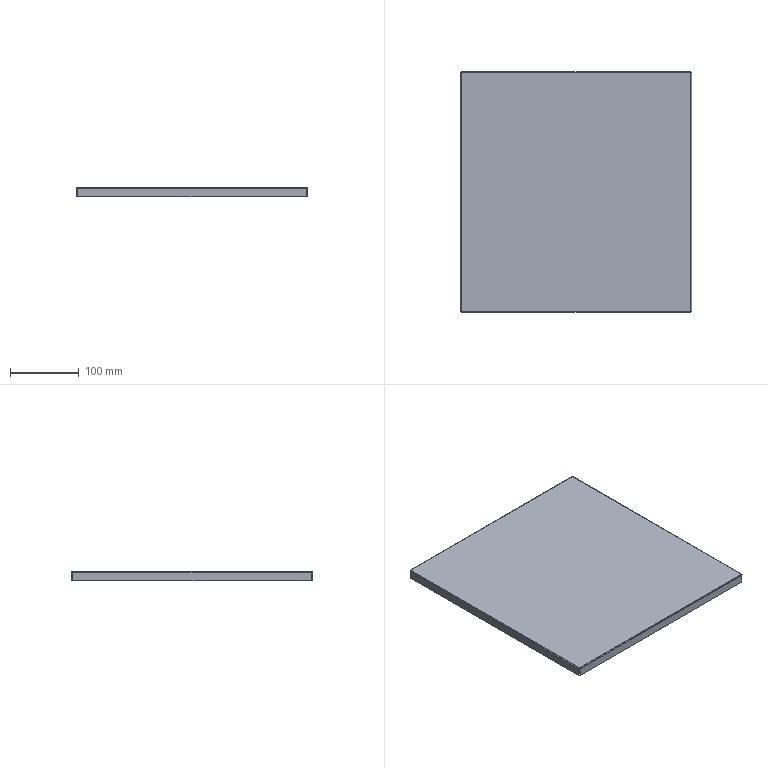Part | STEP file | Electrical plate | 1 solid | 38 faces | box 337.193 x 351.476 x 13.2 mm | volume 161258 mm3 | plane 22 | spline 8 | cylinder 8 | commonest cylinder face diameters 0.4 x4 2.8 x4
STEP:
#1=CARTESIAN_POINT('',(167.196,-174.338,-1.2));
#2=VERTEX_POINT('',#1);
#3=CARTESIAN_POINT('',(167.196,174.338,-1.2));
#4=VERTEX_POINT('',#3);
#5=CARTESIAN_POINT('',(167.196,-174.338,-1.2));
#6=DIRECTION('',(0.,1.,0.));
#7=VECTOR('',#6,1000.);
#8=LINE('',#5,#7);
#9=EDGE_CURVE('',#2,#4,#8,.T.);
#10=ORIENTED_EDGE('',*,*,#9,.F.);
#11=CARTESIAN_POINT('',(-167.196,-174.338,-1.2));
#12=VERTEX_POINT('',#11);
#13=CARTESIAN_POINT('',(-167.196,-174.338,-1.2));
#14=DIRECTION('',(1.,0.,0.));
#15=VECTOR('',#14,1000.);
#16=LINE('',#13,#15);
#17=EDGE_CURVE('',#12,#2,#16,.T.);
#18=ORIENTED_EDGE('',*,*,#17,.F.);
#19=CARTESIAN_POINT('',(-167.196,174.338,-1.2));
#20=VERTEX_POINT('',#19);
#21=CARTESIAN_POINT('',(-167.196,174.338,-1.2));
#22=DIRECTION('',(0.,-1.,0.));
#23=VECTOR('',#22,1000.);
#24=LINE('',#21,#23);
#25=EDGE_CURVE('',#20,#12,#24,.T.);
#26=ORIENTED_EDGE('',*,*,#25,.F.);
#27=CARTESIAN_POINT('',(167.196,174.338,-1.2));
#28=DIRECTION('',(-1.,0.,0.));
#29=VECTOR('',#28,1000.);
#30=LINE('',#27,#29);
#31=EDGE_CURVE('',#4,#20,#30,.T.);
#32=ORIENTED_EDGE('',*,*,#31,.F.);
#33=EDGE_LOOP('',(#10,#18,#26,#32));
#34=FACE_OUTER_BOUND('',#33,.T.);
#35=CARTESIAN_POINT('',(0.,0.,-1.2));
#36=DIRECTION('',(0.,0.,-1.));
#37=DIRECTION('',(-1.,0.,0.));
#38=AXIS2_PLACEMENT_3D('',#35,#36,#37);
#39=PLANE('',#38);
#40=ADVANCED_FACE('',(#34),#39,.T.);
#41=CARTESIAN_POINT('',(-167.196,-174.338,0.));
#42=VERTEX_POINT('',#41);
#43=CARTESIAN_POINT('',(167.196,-174.338,0.));
#44=VERTEX_POINT('',#43);
#45=CARTESIAN_POINT('',(-167.196,-174.338,0.));
#46=DIRECTION('',(1.,0.,0.));
#47=VECTOR('',#46,1000.);
#48=LINE('',#45,#47);
#49=EDGE_CURVE('',#42,#44,#48,.T.);
#50=ORIENTED_EDGE('',*,*,#49,.T.);
#51=CARTESIAN_POINT('',(167.196,174.338,0.));
#52=VERTEX_POINT('',#51);
#53=CARTESIAN_POINT('',(167.196,-174.338,0.));
#54=DIRECTION('',(0.,1.,0.));
#55=VECTOR('',#54,1000.);
#56=LINE('',#53,#55);
#57=EDGE_CURVE('',#44,#52,#56,.T.);
#58=ORIENTED_EDGE('',*,*,#57,.T.);
#59=CARTESIAN_POINT('',(-167.196,174.338,0.));
#60=VERTEX_POINT('',#59);
#61=CARTESIAN_POINT('',(167.196,174.338,0.));
#62=DIRECTION('',(-1.,0.,0.));
#63=VECTOR('',#62,1000.);
#64=LINE('',#61,#63);
#65=EDGE_CURVE('',#52,#60,#64,.T.);
#66=ORIENTED_EDGE('',*,*,#65,.T.);
#67=CARTESIAN_POINT('',(-167.196,174.338,0.));
#68=DIRECTION('',(0.,-1.,0.));
#69=VECTOR('',#68,1000.);
#70=LINE('',#67,#69);
#71=EDGE_CURVE('',#60,#42,#70,.T.);
#72=ORIENTED_EDGE('',*,*,#71,.T.);
#73=EDGE_LOOP('',(#50,#58,#66,#72));
#74=FACE_OUTER_BOUND('',#73,.T.);
#75=CARTESIAN_POINT('',(0.,0.,0.));
#76=DIRECTION('',(0.,0.,-1.));
#77=DIRECTION('',(-1.,0.,0.));
#78=AXIS2_PLACEMENT_3D('',#75,#76,#77);
#79=PLANE('',#78);
#80=ADVANCED_FACE('',(#74),#79,.F.);
#81=CARTESIAN_POINT('',(-168.596,-173.831,-1.4));
#82=VERTEX_POINT('',#81);
#83=CARTESIAN_POINT('',(-167.396,-173.831,-1.4));
#84=VERTEX_POINT('',#83);
#85=CARTESIAN_POINT('',(-167.396,-173.831,-1.4));
#86=DIRECTION('',(1.,0.,0.));
#87=VECTOR('',#86,1000.);
#88=LINE('',#85,#87);
#89=EDGE_CURVE('',#82,#84,#88,.T.);
#90=ORIENTED_EDGE('',*,*,#89,.T.);
#91=CARTESIAN_POINT('',(-167.196,-174.338,-1.2));
#92=CARTESIAN_POINT('',(-167.249,-174.254,-1.2));
#93=CARTESIAN_POINT('',(-167.301,-174.169,-1.222));
#94=CARTESIAN_POINT('',(-167.375,-174.,-1.296));
#95=CARTESIAN_POINT('',(-167.396,-173.916,-1.348));
#96=CARTESIAN_POINT('',(-167.396,-173.831,-1.4));
#97=B_SPLINE_CURVE_WITH_KNOTS('',3,(#91,#92,#93,#94,#95,#96),.UNSPECIFIED.,.F.,.F.,(4,2,4),(0.,0.5,1.),.UNSPECIFIED.);
#98=EDGE_CURVE('',#12,#84,#97,.T.);
#99=ORIENTED_EDGE('',*,*,#98,.F.);
#100=CARTESIAN_POINT('',(-167.196,-174.338,-1.2));
#101=DIRECTION('',(0.,0.,1.));
#102=VECTOR('',#101,1000.);
#103=LINE('',#100,#102);
#104=EDGE_CURVE('',#12,#42,#103,.T.);
#105=ORIENTED_EDGE('',*,*,#104,.T.);
#106=CARTESIAN_POINT('',(-167.196,-174.338,0.));
#107=CARTESIAN_POINT('',(-167.38,-174.296,0.));
#108=CARTESIAN_POINT('',(-167.563,-174.254,-0.03644));
#109=CARTESIAN_POINT('',(-167.901,-174.169,-0.1767));
#110=CARTESIAN_POINT('',(-168.057,-174.127,-0.2805));
#111=CARTESIAN_POINT('',(-168.316,-174.042,-0.5396));
#112=CARTESIAN_POINT('',(-168.42,-174.,-0.6949));
#113=CARTESIAN_POINT('',(-168.56,-173.916,-1.034));
#114=CARTESIAN_POINT('',(-168.596,-173.873,-1.217));
#115=CARTESIAN_POINT('',(-168.596,-173.831,-1.4));
#116=B_SPLINE_CURVE_WITH_KNOTS('',3,(#106,#107,#108,#109,#110,#111,#112,#113,#114,#115),.UNSPECIFIED.,.F.,.F.,(4,2,2,2,4),(0.,0.25,0.5,0.75,1.),.UNSPECIFIED.);
#117=EDGE_CURVE('',#42,#82,#116,.T.);
#118=ORIENTED_EDGE('',*,*,#117,.T.);
#119=EDGE_LOOP('',(#90,#99,#105,#118));
#120=FACE_OUTER_BOUND('',#119,.T.);
#121=CARTESIAN_POINT('',(-167.196,-174.338,0.012));
#122=CARTESIAN_POINT('',(-167.381,-174.296,0.012));
#123=CARTESIAN_POINT('',(-167.566,-174.254,-0.02475));
#124=CARTESIAN_POINT('',(-167.907,-174.169,-0.1662));
#125=CARTESIAN_POINT('',(-168.064,-174.127,-0.2709));
#126=CARTESIAN_POINT('',(-168.325,-174.042,-0.5323));
#127=CARTESIAN_POINT('',(-168.43,-174.,-0.6889));
#128=CARTESIAN_POINT('',(-168.572,-173.916,-1.03));
#129=CARTESIAN_POINT('',(-168.608,-173.873,-1.215));
#130=CARTESIAN_POINT('',(-168.608,-173.831,-1.4));
#131=CARTESIAN_POINT('',(-167.196,-174.338,0.));
#132=CARTESIAN_POINT('',(-167.38,-174.296,0.));
#133=CARTESIAN_POINT('',(-167.563,-174.254,-0.03644));
#134=CARTESIAN_POINT('',(-167.901,-174.169,-0.1767));
#135=CARTESIAN_POINT('',(-168.057,-174.127,-0.2805));
#136=CARTESIAN_POINT('',(-168.316,-174.042,-0.5396));
#137=CARTESIAN_POINT('',(-168.42,-174.,-0.6949));
#138=CARTESIAN_POINT('',(-168.56,-173.916,-1.034));
#139=CARTESIAN_POINT('',(-168.596,-173.873,-1.217));
#140=CARTESIAN_POINT('',(-168.596,-173.831,-1.4));
#141=CARTESIAN_POINT('',(-167.196,-174.338,-1.2));
#142=CARTESIAN_POINT('',(-167.222,-174.296,-1.2));
#143=CARTESIAN_POINT('',(-167.249,-174.254,-1.205));
#144=CARTESIAN_POINT('',(-167.297,-174.169,-1.225));
#145=CARTESIAN_POINT('',(-167.319,-174.127,-1.24));
#146=CARTESIAN_POINT('',(-167.356,-174.042,-1.277));
#147=CARTESIAN_POINT('',(-167.371,-174.,-1.299));
#148=CARTESIAN_POINT('',(-167.391,-173.916,-1.348));
#149=CARTESIAN_POINT('',(-167.396,-173.873,-1.374));
#150=CARTESIAN_POINT('',(-167.396,-173.831,-1.4));
#151=CARTESIAN_POINT('',(-167.196,-174.338,-1.212));
#152=CARTESIAN_POINT('',(-167.221,-174.296,-1.212));
#153=CARTESIAN_POINT('',(-167.245,-174.254,-1.217));
#154=CARTESIAN_POINT('',(-167.291,-174.169,-1.236));
#155=CARTESIAN_POINT('',(-167.312,-174.127,-1.25));
#156=CARTESIAN_POINT('',(-167.347,-174.042,-1.285));
#157=CARTESIAN_POINT('',(-167.36,-174.,-1.305));
#158=CARTESIAN_POINT('',(-167.379,-173.916,-1.351));
#159=CARTESIAN_POINT('',(-167.384,-173.873,-1.375));
#160=CARTESIAN_POINT('',(-167.384,-173.831,-1.4));
#161=B_SPLINE_SURFACE_WITH_KNOTS('',1,3,((#121,#122,#123,#124,#125,#126,#127,#128,#129,#130),(#131,#132,#133,#134,#135,#136,#137,#138,#139,#140),(#141,#142,#143,#144,#145,#146,#147,#148,#149,#150),(#151,#152,#153,#154,#155,#156,#157,#158,#159,#160)),.UNSPECIFIED.,.F.,.F.,.F.,(2,1,1,2),(4,2,2,2,4),(-0.01,0.,1.,1.01),(0.,0.25,0.5,0.75,1.),.UNSPECIFIED.);
#162=ADVANCED_FACE('',(#120),#161,.F.);
#163=CARTESIAN_POINT('',(-167.396,173.831,-1.4));
#164=VERTEX_POINT('',#163);
#165=CARTESIAN_POINT('',(-167.396,173.831,-1.4));
#166=CARTESIAN_POINT('',(-167.396,173.916,-1.348));
#167=CARTESIAN_POINT('',(-167.375,174.,-1.296));
#168=CARTESIAN_POINT('',(-167.301,174.169,-1.222));
#169=CARTESIAN_POINT('',(-167.249,174.254,-1.2));
#170=CARTESIAN_POINT('',(-167.196,174.338,-1.2));
#171=B_SPLINE_CURVE_WITH_KNOTS('',3,(#165,#166,#167,#168,#169,#170),.UNSPECIFIED.,.F.,.F.,(4,2,4),(0.,0.5,1.),.UNSPECIFIED.);
#172=EDGE_CURVE('',#164,#20,#171,.T.);
#173=ORIENTED_EDGE('',*,*,#172,.F.);
#174=CARTESIAN_POINT('',(-168.596,173.831,-1.4));
#175=VERTEX_POINT('',#174);
#176=CARTESIAN_POINT('',(-167.396,173.831,-1.4));
#177=DIRECTION('',(1.,0.,0.));
#178=VECTOR('',#177,1000.);
#179=LINE('',#176,#178);
#180=EDGE_CURVE('',#175,#164,#179,.T.);
#181=ORIENTED_EDGE('',*,*,#180,.F.);
#182=CARTESIAN_POINT('',(-168.596,173.831,-1.4));
#183=CARTESIAN_POINT('',(-168.596,173.873,-1.217));
#184=CARTESIAN_POINT('',(-168.56,173.916,-1.034));
#185=CARTESIAN_POINT('',(-168.42,174.,-0.6949));
#186=CARTESIAN_POINT('',(-168.316,174.042,-0.5396));
#187=CARTESIAN_POINT('',(-168.057,174.127,-0.2805));
#188=CARTESIAN_POINT('',(-167.901,174.169,-0.1767));
#189=CARTESIAN_POINT('',(-167.563,174.254,-0.03644));
#190=CARTESIAN_POINT('',(-167.38,174.296,0.));
#191=CARTESIAN_POINT('',(-167.196,174.338,0.));
#192=B_SPLINE_CURVE_WITH_KNOTS('',3,(#182,#183,#184,#185,#186,#187,#188,#189,#190,#191),.UNSPECIFIED.,.F.,.F.,(4,2,2,2,4),(0.,0.25,0.5,0.75,1.),.UNSPECIFIED.);
#193=EDGE_CURVE('',#175,#60,#192,.T.);
#194=ORIENTED_EDGE('',*,*,#193,.T.);
#195=CARTESIAN_POINT('',(-167.196,174.338,-1.2));
#196=DIRECTION('',(0.,0.,1.));
#197=VECTOR('',#196,1000.);
#198=LINE('',#195,#197);
#199=EDGE_CURVE('',#20,#60,#198,.T.);
#200=ORIENTED_EDGE('',*,*,#199,.F.);
#201=EDGE_LOOP('',(#173,#181,#194,#200));
#202=FACE_OUTER_BOUND('',#201,.T.);
#203=CARTESIAN_POINT('',(-168.608,173.831,-1.4));
#204=CARTESIAN_POINT('',(-168.608,173.873,-1.215));
#205=CARTESIAN_POINT('',(-168.572,173.916,-1.03));
#206=CARTESIAN_POINT('',(-168.43,174.,-0.6889));
#207=CARTESIAN_POINT('',(-168.325,174.042,-0.5323));
#208=CARTESIAN_POINT('',(-168.064,174.127,-0.2709));
#209=CARTESIAN_POINT('',(-167.907,174.169,-0.1662));
#210=CARTESIAN_POINT('',(-167.566,174.254,-0.02475));
#211=CARTESIAN_POINT('',(-167.381,174.296,0.012));
#212=CARTESIAN_POINT('',(-167.196,174.338,0.012));
#213=CARTESIAN_POINT('',(-168.596,173.831,-1.4));
#214=CARTESIAN_POINT('',(-168.596,173.873,-1.217));
#215=CARTESIAN_POINT('',(-168.56,173.916,-1.034));
#216=CARTESIAN_POINT('',(-168.42,174.,-0.6949));
#217=CARTESIAN_POINT('',(-168.316,174.042,-0.5396));
#218=CARTESIAN_POINT('',(-168.057,174.127,-0.2805));
#219=CARTESIAN_POINT('',(-167.901,174.169,-0.1767));
#220=CARTESIAN_POINT('',(-167.563,174.254,-0.03644));
#221=CARTESIAN_POINT('',(-167.38,174.296,0.));
#222=CARTESIAN_POINT('',(-167.196,174.338,0.));
#223=CARTESIAN_POINT('',(-167.396,173.831,-1.4));
#224=CARTESIAN_POINT('',(-167.396,173.873,-1.374));
#225=CARTESIAN_POINT('',(-167.391,173.916,-1.348));
#226=CARTESIAN_POINT('',(-167.371,174.,-1.299));
#227=CARTESIAN_POINT('',(-167.356,174.042,-1.277));
#228=CARTESIAN_POINT('',(-167.319,174.127,-1.24));
#229=CARTESIAN_POINT('',(-167.297,174.169,-1.225));
#230=CARTESIAN_POINT('',(-167.249,174.254,-1.205));
#231=CARTESIAN_POINT('',(-167.222,174.296,-1.2));
#232=CARTESIAN_POINT('',(-167.196,174.338,-1.2));
#233=CARTESIAN_POINT('',(-167.384,173.831,-1.4));
#234=CARTESIAN_POINT('',(-167.384,173.873,-1.375));
#235=CARTESIAN_POINT('',(-167.379,173.916,-1.351));
#236=CARTESIAN_POINT('',(-167.36,174.,-1.305));
#237=CARTESIAN_POINT('',(-167.347,174.042,-1.285));
#238=CARTESIAN_POINT('',(-167.312,174.127,-1.25));
#239=CARTESIAN_POINT('',(-167.291,174.169,-1.236));
#240=CARTESIAN_POINT('',(-167.245,174.254,-1.217));
#241=CARTESIAN_POINT('',(-167.221,174.296,-1.212));
#242=CARTESIAN_POINT('',(-167.196,174.338,-1.212));
#243=B_SPLINE_SURFACE_WITH_KNOTS('',1,3,((#203,#204,#205,#206,#207,#208,#209,#210,#211,#212),(#213,#214,#215,#216,#217,#218,#219,#220,#221,#222),(#223,#224,#225,#226,#227,#228,#229,#230,#231,#232),(#233,#234,#235,#236,#237,#238,#239,#240,#241,#242)),.UNSPECIFIED.,.F.,.F.,.F.,(2,1,1,2),(4,2,2,2,4),(-0.01,0.,1.,1.01),(0.,0.25,0.5,0.75,1.),.UNSPECIFIED.);
#244=ADVANCED_FACE('',(#202),#243,.F.);
#245=ORIENTED_EDGE('',*,*,#71,.F.);
#246=ORIENTED_EDGE('',*,*,#193,.F.);
#247=CARTESIAN_POINT('',(-168.596,0.,-1.4));
#248=DIRECTION('',(0.,1.,0.));
#249=VECTOR('',#248,1000.);
#250=LINE('',#247,#249);
#251=EDGE_CURVE('',#82,#175,#250,.T.);
#252=ORIENTED_EDGE('',*,*,#251,.F.);
#253=ORIENTED_EDGE('',*,*,#117,.F.);
#254=EDGE_LOOP('',(#245,#246,#252,#253));
#255=FACE_OUTER_BOUND('',#254,.T.);
#256=CARTESIAN_POINT('',(-167.196,174.338,-1.4));
#257=DIRECTION('',(0.,1.,0.));
#258=DIRECTION('',(-1.,0.,0.));
#259=AXIS2_PLACEMENT_3D('',#256,#257,#258);
#260=CYLINDRICAL_SURFACE('',#259,1.4);
#261=ADVANCED_FACE('',(#255),#260,.T.);
#262=ORIENTED_EDGE('',*,*,#25,.T.);
#263=ORIENTED_EDGE('',*,*,#98,.T.);
#264=CARTESIAN_POINT('',(-167.396,-174.538,-1.4));
#265=DIRECTION('',(0.,1.,0.));
#266=VECTOR('',#265,1000.);
#267=LINE('',#264,#266);
#268=EDGE_CURVE('',#84,#164,#267,.T.);
#269=ORIENTED_EDGE('',*,*,#268,.T.);
#270=ORIENTED_EDGE('',*,*,#172,.T.);
#271=EDGE_LOOP('',(#262,#263,#269,#270));
#272=FACE_OUTER_BOUND('',#271,.T.);
#273=CARTESIAN_POINT('',(-167.196,174.338,-1.4));
#274=DIRECTION('',(0.,1.,0.));
#275=DIRECTION('',(-1.,0.,0.));
#276=AXIS2_PLACEMENT_3D('',#273,#274,#275);
#277=CYLINDRICAL_SURFACE('',#276,0.2);
#278=ADVANCED_FACE('',(#272),#277,.F.);
#279=CARTESIAN_POINT('',(-167.396,-173.831,-13.2));
#280=VERTEX_POINT('',#279);
#281=CARTESIAN_POINT('',(-168.596,-173.831,-13.2));
#282=VERTEX_POINT('',#281);
#283=CARTESIAN_POINT('',(-168.596,-173.831,-13.2));
#284=DIRECTION('',(-1.,0.,0.));
#285=VECTOR('',#284,1000.);
#286=LINE('',#283,#285);
#287=EDGE_CURVE('',#280,#282,#286,.T.);
#288=ORIENTED_EDGE('',*,*,#287,.F.);
#289=CARTESIAN_POINT('',(-167.396,-173.831,-1.2));
#290=DIRECTION('',(0.,0.,-1.));
#291=VECTOR('',#290,1000.);
#292=LINE('',#289,#291);
#293=EDGE_CURVE('',#84,#280,#292,.T.);
#294=ORIENTED_EDGE('',*,*,#293,.F.);
#295=ORIENTED_EDGE('',*,*,#89,.F.);
#296=CARTESIAN_POINT('',(-168.596,-173.831,0.));
#297=DIRECTION('',(0.,0.,1.));
#298=VECTOR('',#297,1000.);
#299=LINE('',#296,#298);
#300=EDGE_CURVE('',#282,#82,#299,.T.);
#301=ORIENTED_EDGE('',*,*,#300,.F.);
#302=EDGE_LOOP('',(#288,#294,#295,#301));
#303=FACE_OUTER_BOUND('',#302,.T.);
#304=CARTESIAN_POINT('',(-167.396,-173.831,-1.2));
#305=DIRECTION('',(0.,-1.,0.));
#306=DIRECTION('',(0.,0.,-1.));
#307=AXIS2_PLACEMENT_3D('',#304,#305,#306);
#308=PLANE('',#307);
#309=ADVANCED_FACE('',(#303),#308,.T.);
#310=CARTESIAN_POINT('',(-168.596,173.831,-13.2));
#311=VERTEX_POINT('',#310);
#312=CARTESIAN_POINT('',(-168.596,173.831,0.));
#313=DIRECTION('',(0.,0.,1.));
#314=VECTOR('',#313,1000.);
#315=LINE('',#312,#314);
#316=EDGE_CURVE('',#311,#175,#315,.T.);
#317=ORIENTED_EDGE('',*,*,#316,.F.);
#318=CARTESIAN_POINT('',(-168.596,174.538,-13.2));
#319=DIRECTION('',(0.,1.,0.));
#320=VECTOR('',#319,1000.);
#321=LINE('',#318,#320);
#322=EDGE_CURVE('',#282,#311,#321,.T.);
#323=ORIENTED_EDGE('',*,*,#322,.F.);
#324=ORIENTED_EDGE('',*,*,#300,.T.);
#325=ORIENTED_EDGE('',*,*,#251,.T.);
#326=EDGE_LOOP('',(#317,#323,#324,#325));
#327=FACE_OUTER_BOUND('',#326,.T.);
#328=CARTESIAN_POINT('',(-168.596,0.,0.));
#329=DIRECTION('',(-1.,0.,0.));
#330=DIRECTION('',(0.,0.,1.));
#331=AXIS2_PLACEMENT_3D('',#328,#329,#330);
#332=PLANE('',#331);
#333=ADVANCED_FACE('',(#327),#332,.T.);
#334=CARTESIAN_POINT('',(-167.396,173.831,-13.2));
#335=VERTEX_POINT('',#334);
#336=CARTESIAN_POINT('',(-167.396,174.538,-13.2));
#337=DIRECTION('',(0.,1.,0.));
#338=VECTOR('',#337,1000.);
#339=LINE('',#336,#338);
#340=EDGE_CURVE('',#280,#335,#339,.T.);
#341=ORIENTED_EDGE('',*,*,#340,.T.);
#342=CARTESIAN_POINT('',(-167.396,173.831,-1.2));
#343=DIRECTION('',(0.,0.,-1.));
#344=VECTOR('',#343,1000.);
#345=LINE('',#342,#344);
#346=EDGE_CURVE('',#164,#335,#345,.T.);
#347=ORIENTED_EDGE('',*,*,#346,.F.);
#348=ORIENTED_EDGE('',*,*,#268,.F.);
#349=ORIENTED_EDGE('',*,*,#293,.T.);
#350=EDGE_LOOP('',(#341,#347,#348,#349));
#351=FACE_OUTER_BOUND('',#350,.T.);
#352=CARTESIAN_POINT('',(-167.396,0.,0.));
#353=DIRECTION('',(-1.,0.,0.));
#354=DIRECTION('',(0.,0.,1.));
#355=AXIS2_PLACEMENT_3D('',#352,#353,#354);
#356=PLANE('',#355);
#357=ADVANCED_FACE('',(#351),#356,.F.);
#358=CARTESIAN_POINT('',(-168.596,173.831,-13.2));
#359=DIRECTION('',(-1.,0.,0.));
#360=VECTOR('',#359,1000.);
#361=LINE('',#358,#360);
#362=EDGE_CURVE('',#335,#311,#361,.T.);
#363=ORIENTED_EDGE('',*,*,#362,.F.);
#364=ORIENTED_EDGE('',*,*,#340,.F.);
#365=ORIENTED_EDGE('',*,*,#287,.T.);
#366=ORIENTED_EDGE('',*,*,#322,.T.);
#367=EDGE_LOOP('',(#363,#364,#365,#366));
#368=FACE_OUTER_BOUND('',#367,.T.);
#369=CARTESIAN_POINT('',(-168.596,174.538,-13.2));
#370=DIRECTION('',(0.,0.,-1.));
#371=DIRECTION('',(-1.,0.,0.));
#372=AXIS2_PLACEMENT_3D('',#369,#370,#371);
#373=PLANE('',#372);
#374=ADVANCED_FACE('',(#368),#373,.T.);
#375=ORIENTED_EDGE('',*,*,#346,.T.);
#376=ORIENTED_EDGE('',*,*,#362,.T.);
#377=ORIENTED_EDGE('',*,*,#316,.T.);
#378=ORIENTED_EDGE('',*,*,#180,.T.);
#379=EDGE_LOOP('',(#375,#376,#377,#378));
#380=FACE_OUTER_BOUND('',#379,.T.);
#381=CARTESIAN_POINT('',(-167.396,173.831,-1.2));
#382=DIRECTION('',(0.,-1.,0.));
#383=DIRECTION('',(0.,0.,-1.));
#384=AXIS2_PLACEMENT_3D('',#381,#382,#383);
#385=PLANE('',#384);
#386=ADVANCED_FACE('',(#380),#385,.F.);
#387=CARTESIAN_POINT('',(-166.689,175.738,-1.4));
#388=VERTEX_POINT('',#387);
#389=CARTESIAN_POINT('',(-166.689,174.538,-1.4));
#390=VERTEX_POINT('',#389);
#391=CARTESIAN_POINT('',(-166.689,174.538,-1.4));
#392=DIRECTION('',(0.,-1.,0.));
#393=VECTOR('',#392,1000.);
#394=LINE('',#391,#393);
#395=EDGE_CURVE('',#388,#390,#394,.T.);
#396=ORIENTED_EDGE('',*,*,#395,.T.);
#397=CARTESIAN_POINT('',(-167.196,174.338,-1.2));
#398=CARTESIAN_POINT('',(-167.112,174.39,-1.2));
#399=CARTESIAN_POINT('',(-167.027,174.443,-1.222));
#400=CARTESIAN_POINT('',(-166.858,174.517,-1.296));
#401=CARTESIAN_POINT('',(-166.774,174.538,-1.348));
#402=CARTESIAN_POINT('',(-166.689,174.538,-1.4));
#403=B_SPLINE_CURVE_WITH_KNOTS('',3,(#397,#398,#399,#400,#401,#402),.UNSPECIFIED.,.F.,.F.,(4,2,4),(0.,0.5,1.),.UNSPECIFIED.);
#404=EDGE_CURVE('',#20,#390,#403,.T.);
#405=ORIENTED_EDGE('',*,*,#404,.F.);
#406=ORIENTED_EDGE('',*,*,#199,.T.);
#407=CARTESIAN_POINT('',(-167.196,174.338,0.));
#408=CARTESIAN_POINT('',(-167.154,174.521,0.));
#409=CARTESIAN_POINT('',(-167.112,174.705,-0.03644));
#410=CARTESIAN_POINT('',(-167.027,175.043,-0.1767));
#411=CARTESIAN_POINT('',(-166.985,175.198,-0.2805));
#412=CARTESIAN_POINT('',(-166.9,175.458,-0.5396));
#413=CARTESIAN_POINT('',(-166.858,175.561,-0.6949));
#414=CARTESIAN_POINT('',(-166.774,175.702,-1.034));
#415=CARTESIAN_POINT('',(-166.731,175.738,-1.217));
#416=CARTESIAN_POINT('',(-166.689,175.738,-1.4));
#417=B_SPLINE_CURVE_WITH_KNOTS('',3,(#407,#408,#409,#410,#411,#412,#413,#414,#415,#416),.UNSPECIFIED.,.F.,.F.,(4,2,2,2,4),(0.,0.25,0.5,0.75,1.),.UNSPECIFIED.);
#418=EDGE_CURVE('',#60,#388,#417,.T.);
#419=ORIENTED_EDGE('',*,*,#418,.T.);
#420=EDGE_LOOP('',(#396,#405,#406,#419));
#421=FACE_OUTER_BOUND('',#420,.T.);
#422=CARTESIAN_POINT('',(-167.196,174.338,0.012));
#423=CARTESIAN_POINT('',(-167.154,174.523,0.012));
#424=CARTESIAN_POINT('',(-167.112,174.708,-0.02475));
#425=CARTESIAN_POINT('',(-167.027,175.049,-0.1662));
#426=CARTESIAN_POINT('',(-166.985,175.206,-0.2709));
#427=CARTESIAN_POINT('',(-166.9,175.467,-0.5323));
#428=CARTESIAN_POINT('',(-166.858,175.572,-0.6889));
#429=CARTESIAN_POINT('',(-166.774,175.713,-1.03));
#430=CARTESIAN_POINT('',(-166.731,175.75,-1.215));
#431=CARTESIAN_POINT('',(-166.689,175.75,-1.4));
#432=CARTESIAN_POINT('',(-167.196,174.338,0.));
#433=CARTESIAN_POINT('',(-167.154,174.521,0.));
#434=CARTESIAN_POINT('',(-167.112,174.705,-0.03644));
#435=CARTESIAN_POINT('',(-167.027,175.043,-0.1767));
#436=CARTESIAN_POINT('',(-166.985,175.198,-0.2805));
#437=CARTESIAN_POINT('',(-166.9,175.458,-0.5396));
#438=CARTESIAN_POINT('',(-166.858,175.561,-0.6949));
#439=CARTESIAN_POINT('',(-166.774,175.702,-1.034));
#440=CARTESIAN_POINT('',(-166.731,175.738,-1.217));
#441=CARTESIAN_POINT('',(-166.689,175.738,-1.4));
#442=CARTESIAN_POINT('',(-167.196,174.338,-1.2));
#443=CARTESIAN_POINT('',(-167.154,174.364,-1.2));
#444=CARTESIAN_POINT('',(-167.112,174.39,-1.205));
#445=CARTESIAN_POINT('',(-167.027,174.439,-1.225));
#446=CARTESIAN_POINT('',(-166.985,174.461,-1.24));
#447=CARTESIAN_POINT('',(-166.9,174.498,-1.277));
#448=CARTESIAN_POINT('',(-166.858,174.513,-1.299));
#449=CARTESIAN_POINT('',(-166.774,174.533,-1.348));
#450=CARTESIAN_POINT('',(-166.731,174.538,-1.374));
#451=CARTESIAN_POINT('',(-166.689,174.538,-1.4));
#452=CARTESIAN_POINT('',(-167.196,174.338,-1.212));
#453=CARTESIAN_POINT('',(-167.154,174.363,-1.212));
#454=CARTESIAN_POINT('',(-167.112,174.387,-1.217));
#455=CARTESIAN_POINT('',(-167.027,174.433,-1.236));
#456=CARTESIAN_POINT('',(-166.985,174.454,-1.25));
#457=CARTESIAN_POINT('',(-166.9,174.488,-1.285));
#458=CARTESIAN_POINT('',(-166.858,174.502,-1.305));
#459=CARTESIAN_POINT('',(-166.774,174.521,-1.351));
#460=CARTESIAN_POINT('',(-166.731,174.526,-1.375));
#461=CARTESIAN_POINT('',(-166.689,174.526,-1.4));
#462=B_SPLINE_SURFACE_WITH_KNOTS('',1,3,((#422,#423,#424,#425,#426,#427,#428,#429,#430,#431),(#432,#433,#434,#435,#436,#437,#438,#439,#440,#441),(#442,#443,#444,#445,#446,#447,#448,#449,#450,#451),(#452,#453,#454,#455,#456,#457,#458,#459,#460,#461)),.UNSPECIFIED.,.F.,.F.,.F.,(2,1,1,2),(4,2,2,2,4),(-0.01,0.,1.,1.01),(0.,0.25,0.5,0.75,1.),.UNSPECIFIED.);
#463=ADVANCED_FACE('',(#421),#462,.F.);
#464=CARTESIAN_POINT('',(166.689,174.538,-1.4));
#465=VERTEX_POINT('',#464);
#466=CARTESIAN_POINT('',(166.689,174.538,-1.4));
#467=CARTESIAN_POINT('',(166.774,174.538,-1.348));
#468=CARTESIAN_POINT('',(166.858,174.517,-1.296));
#469=CARTESIAN_POINT('',(167.027,174.443,-1.222));
#470=CARTESIAN_POINT('',(167.112,174.39,-1.2));
#471=CARTESIAN_POINT('',(167.196,174.338,-1.2));
#472=B_SPLINE_CURVE_WITH_KNOTS('',3,(#466,#467,#468,#469,#470,#471),.UNSPECIFIED.,.F.,.F.,(4,2,4),(0.,0.5,1.),.UNSPECIFIED.);
#473=EDGE_CURVE('',#465,#4,#472,.T.);
#474=ORIENTED_EDGE('',*,*,#473,.F.);
#475=CARTESIAN_POINT('',(166.689,175.738,-1.4));
#476=VERTEX_POINT('',#475);
#477=CARTESIAN_POINT('',(166.689,174.538,-1.4));
#478=DIRECTION('',(0.,-1.,0.));
#479=VECTOR('',#478,1000.);
#480=LINE('',#477,#479);
#481=EDGE_CURVE('',#476,#465,#480,.T.);
#482=ORIENTED_EDGE('',*,*,#481,.F.);
#483=CARTESIAN_POINT('',(166.689,175.738,-1.4));
#484=CARTESIAN_POINT('',(166.731,175.738,-1.217));
#485=CARTESIAN_POINT('',(166.774,175.702,-1.034));
#486=CARTESIAN_POINT('',(166.858,175.561,-0.6949));
#487=CARTESIAN_POINT('',(166.9,175.458,-0.5396));
#488=CARTESIAN_POINT('',(166.985,175.198,-0.2805));
#489=CARTESIAN_POINT('',(167.027,175.043,-0.1767));
#490=CARTESIAN_POINT('',(167.112,174.705,-0.03644));
#491=CARTESIAN_POINT('',(167.154,174.521,0.));
#492=CARTESIAN_POINT('',(167.196,174.338,0.));
#493=B_SPLINE_CURVE_WITH_KNOTS('',3,(#483,#484,#485,#486,#487,#488,#489,#490,#491,#492),.UNSPECIFIED.,.F.,.F.,(4,2,2,2,4),(0.,0.25,0.5,0.75,1.),.UNSPECIFIED.);
#494=EDGE_CURVE('',#476,#52,#493,.T.);
#495=ORIENTED_EDGE('',*,*,#494,.T.);
#496=CARTESIAN_POINT('',(167.196,174.338,-1.2));
#497=DIRECTION('',(0.,0.,1.));
#498=VECTOR('',#497,1000.);
#499=LINE('',#496,#498);
#500=EDGE_CURVE('',#4,#52,#499,.T.);
#501=ORIENTED_EDGE('',*,*,#500,.F.);
#502=EDGE_LOOP('',(#474,#482,#495,#501));
#503=FACE_OUTER_BOUND('',#502,.T.);
#504=CARTESIAN_POINT('',(166.689,175.75,-1.4));
#505=CARTESIAN_POINT('',(166.731,175.75,-1.215));
#506=CARTESIAN_POINT('',(166.774,175.713,-1.03));
#507=CARTESIAN_POINT('',(166.858,175.572,-0.6889));
#508=CARTESIAN_POINT('',(166.9,175.467,-0.5323));
#509=CARTESIAN_POINT('',(166.985,175.206,-0.2709));
#510=CARTESIAN_POINT('',(167.027,175.049,-0.1662));
#511=CARTESIAN_POINT('',(167.112,174.708,-0.02475));
#512=CARTESIAN_POINT('',(167.154,174.523,0.012));
#513=CARTESIAN_POINT('',(167.196,174.338,0.012));
#514=CARTESIAN_POINT('',(166.689,175.738,-1.4));
#515=CARTESIAN_POINT('',(166.731,175.738,-1.217));
#516=CARTESIAN_POINT('',(166.774,175.702,-1.034));
#517=CARTESIAN_POINT('',(166.858,175.561,-0.6949));
#518=CARTESIAN_POINT('',(166.9,175.458,-0.5396));
#519=CARTESIAN_POINT('',(166.985,175.198,-0.2805));
#520=CARTESIAN_POINT('',(167.027,175.043,-0.1767));
#521=CARTESIAN_POINT('',(167.112,174.705,-0.03644));
#522=CARTESIAN_POINT('',(167.154,174.521,0.));
#523=CARTESIAN_POINT('',(167.196,174.338,0.));
#524=CARTESIAN_POINT('',(166.689,174.538,-1.4));
#525=CARTESIAN_POINT('',(166.731,174.538,-1.374));
#526=CARTESIAN_POINT('',(166.774,174.533,-1.348));
#527=CARTESIAN_POINT('',(166.858,174.513,-1.299));
#528=CARTESIAN_POINT('',(166.9,174.498,-1.277));
#529=CARTESIAN_POINT('',(166.985,174.461,-1.24));
#530=CARTESIAN_POINT('',(167.027,174.439,-1.225));
#531=CARTESIAN_POINT('',(167.112,174.39,-1.205));
#532=CARTESIAN_POINT('',(167.154,174.364,-1.2));
#533=CARTESIAN_POINT('',(167.196,174.338,-1.2));
#534=CARTESIAN_POINT('',(166.689,174.526,-1.4));
#535=CARTESIAN_POINT('',(166.731,174.526,-1.375));
#536=CARTESIAN_POINT('',(166.774,174.521,-1.351));
#537=CARTESIAN_POINT('',(166.858,174.502,-1.305));
#538=CARTESIAN_POINT('',(166.9,174.488,-1.285));
#539=CARTESIAN_POINT('',(166.985,174.454,-1.25));
#540=CARTESIAN_POINT('',(167.027,174.433,-1.236));
#541=CARTESIAN_POINT('',(167.112,174.387,-1.217));
#542=CARTESIAN_POINT('',(167.154,174.363,-1.212));
#543=CARTESIAN_POINT('',(167.196,174.338,-1.212));
#544=B_SPLINE_SURFACE_WITH_KNOTS('',1,3,((#504,#505,#506,#507,#508,#509,#510,#511,#512,#513),(#514,#515,#516,#517,#518,#519,#520,#521,#522,#523),(#524,#525,#526,#527,#528,#529,#530,#531,#532,#533),(#534,#535,#536,#537,#538,#539,#540,#541,#542,#543)),.UNSPECIFIED.,.F.,.F.,.F.,(2,1,1,2),(4,2,2,2,4),(-0.01,0.,1.,1.01),(0.,0.25,0.5,0.75,1.),.UNSPECIFIED.);
#545=ADVANCED_FACE('',(#503),#544,.F.);
#546=ORIENTED_EDGE('',*,*,#65,.F.);
#547=ORIENTED_EDGE('',*,*,#494,.F.);
#548=CARTESIAN_POINT('',(0.,175.738,-1.4));
#549=DIRECTION('',(-1.,0.,0.));
#550=VECTOR('',#549,1000.);
#551=LINE('',#548,#550);
#552=EDGE_CURVE('',#476,#388,#551,.T.);
#553=ORIENTED_EDGE('',*,*,#552,.T.);
#554=ORIENTED_EDGE('',*,*,#418,.F.);
#555=EDGE_LOOP('',(#546,#547,#553,#554));
#556=FACE_OUTER_BOUND('',#555,.T.);
#557=CARTESIAN_POINT('',(167.196,174.338,-1.4));
#558=DIRECTION('',(1.,0.,0.));
#559=DIRECTION('',(0.,1.,0.));
#560=AXIS2_PLACEMENT_3D('',#557,#558,#559);
#561=CYLINDRICAL_SURFACE('',#560,1.4);
#562=ADVANCED_FACE('',(#556),#561,.T.);
#563=ORIENTED_EDGE('',*,*,#31,.T.);
#564=ORIENTED_EDGE('',*,*,#404,.T.);
#565=CARTESIAN_POINT('',(-167.396,174.538,-1.4));
#566=DIRECTION('',(1.,0.,0.));
#567=VECTOR('',#566,1000.);
#568=LINE('',#565,#567);
#569=EDGE_CURVE('',#390,#465,#568,.T.);
#570=ORIENTED_EDGE('',*,*,#569,.T.);
#571=ORIENTED_EDGE('',*,*,#473,.T.);
#572=EDGE_LOOP('',(#563,#564,#570,#571));
#573=FACE_OUTER_BOUND('',#572,.T.);
#574=CARTESIAN_POINT('',(167.196,174.338,-1.4));
#575=DIRECTION('',(1.,0.,0.));
#576=DIRECTION('',(0.,1.,0.));
#577=AXIS2_PLACEMENT_3D('',#574,#575,#576);
#578=CYLINDRICAL_SURFACE('',#577,0.2);
#579=ADVANCED_FACE('',(#573),#578,.F.);
#580=CARTESIAN_POINT('',(-166.689,174.538,-13.2));
#581=VERTEX_POINT('',#580);
#582=CARTESIAN_POINT('',(-166.689,175.738,-13.2));
#583=VERTEX_POINT('',#582);
#584=CARTESIAN_POINT('',(-166.689,175.738,-13.2));
#585=DIRECTION('',(0.,1.,0.));
#586=VECTOR('',#585,1000.);
#587=LINE('',#584,#586);
#588=EDGE_CURVE('',#581,#583,#587,.T.);
#589=ORIENTED_EDGE('',*,*,#588,.F.);
#590=CARTESIAN_POINT('',(-166.689,174.538,-1.2));
#591=DIRECTION('',(0.,0.,-1.));
#592=VECTOR('',#591,1000.);
#593=LINE('',#590,#592);
#594=EDGE_CURVE('',#390,#581,#593,.T.);
#595=ORIENTED_EDGE('',*,*,#594,.F.);
#596=ORIENTED_EDGE('',*,*,#395,.F.);
#597=CARTESIAN_POINT('',(-166.689,175.738,0.));
#598=DIRECTION('',(0.,0.,-1.));
#599=VECTOR('',#598,1000.);
#600=LINE('',#597,#599);
#601=EDGE_CURVE('',#388,#583,#600,.T.);
#602=ORIENTED_EDGE('',*,*,#601,.T.);
#603=EDGE_LOOP('',(#589,#595,#596,#602));
#604=FACE_OUTER_BOUND('',#603,.T.);
#605=CARTESIAN_POINT('',(-166.689,174.538,-1.2));
#606=DIRECTION('',(-1.,0.,0.));
#607=DIRECTION('',(0.,0.,1.));
#608=AXIS2_PLACEMENT_3D('',#605,#606,#607);
#609=PLANE('',#608);
#610=ADVANCED_FACE('',(#604),#609,.T.);
#611=ORIENTED_EDGE('',*,*,#552,.F.);
#612=CARTESIAN_POINT('',(166.689,175.738,-13.2));
#613=VERTEX_POINT('',#612);
#614=CARTESIAN_POINT('',(166.689,175.738,0.));
#615=DIRECTION('',(0.,0.,-1.));
#616=VECTOR('',#615,1000.);
#617=LINE('',#614,#616);
#618=EDGE_CURVE('',#476,#613,#617,.T.);
#619=ORIENTED_EDGE('',*,*,#618,.T.);
#620=CARTESIAN_POINT('',(-167.396,175.738,-13.2));
#621=DIRECTION('',(1.,0.,0.));
#622=VECTOR('',#621,1000.);
#623=LINE('',#620,#622);
#624=EDGE_CURVE('',#583,#613,#623,.T.);
#625=ORIENTED_EDGE('',*,*,#624,.F.);
#626=ORIENTED_EDGE('',*,*,#601,.F.);
#627=EDGE_LOOP('',(#611,#619,#625,#626));
#628=FACE_OUTER_BOUND('',#627,.T.);
#629=CARTESIAN_POINT('',(0.,175.738,0.));
#630=DIRECTION('',(0.,-1.,0.));
#631=DIRECTION('',(0.,0.,-1.));
#632=AXIS2_PLACEMENT_3D('',#629,#630,#631);
#633=PLANE('',#632);
#634=ADVANCED_FACE('',(#628),#633,.F.);
#635=CARTESIAN_POINT('',(166.689,174.538,-13.2));
#636=VERTEX_POINT('',#635);
#637=CARTESIAN_POINT('',(166.689,174.538,-1.2));
#638=DIRECTION('',(0.,0.,-1.));
#639=VECTOR('',#638,1000.);
#640=LINE('',#637,#639);
#641=EDGE_CURVE('',#465,#636,#640,.T.);
#642=ORIENTED_EDGE('',*,*,#641,.F.);
#643=ORIENTED_EDGE('',*,*,#569,.F.);
#644=ORIENTED_EDGE('',*,*,#594,.T.);
#645=CARTESIAN_POINT('',(-167.396,174.538,-13.2));
#646=DIRECTION('',(1.,0.,0.));
#647=VECTOR('',#646,1000.);
#648=LINE('',#645,#647);
#649=EDGE_CURVE('',#581,#636,#648,.T.);
#650=ORIENTED_EDGE('',*,*,#649,.T.);
#651=EDGE_LOOP('',(#642,#643,#644,#650));
#652=FACE_OUTER_BOUND('',#651,.T.);
#653=CARTESIAN_POINT('',(0.,174.538,0.));
#654=DIRECTION('',(0.,-1.,0.));
#655=DIRECTION('',(0.,0.,-1.));
#656=AXIS2_PLACEMENT_3D('',#653,#654,#655);
#657=PLANE('',#656);
#658=ADVANCED_FACE('',(#652),#657,.T.);
#659=CARTESIAN_POINT('',(166.689,175.738,-13.2));
#660=DIRECTION('',(0.,1.,0.));
#661=VECTOR('',#660,1000.);
#662=LINE('',#659,#661);
#663=EDGE_CURVE('',#636,#613,#662,.T.);
#664=ORIENTED_EDGE('',*,*,#663,.F.);
#665=ORIENTED_EDGE('',*,*,#649,.F.);
#666=ORIENTED_EDGE('',*,*,#588,.T.);
#667=ORIENTED_EDGE('',*,*,#624,.T.);
#668=EDGE_LOOP('',(#664,#665,#666,#667));
#669=FACE_OUTER_BOUND('',#668,.T.);
#670=CARTESIAN_POINT('',(-167.396,175.738,-13.2));
#671=DIRECTION('',(0.,0.,-1.));
#672=DIRECTION('',(0.,1.,0.));
#673=AXIS2_PLACEMENT_3D('',#670,#671,#672);
#674=PLANE('',#673);
#675=ADVANCED_FACE('',(#669),#674,.T.);
#676=ORIENTED_EDGE('',*,*,#641,.T.);
#677=ORIENTED_EDGE('',*,*,#663,.T.);
#678=ORIENTED_EDGE('',*,*,#618,.F.);
#679=ORIENTED_EDGE('',*,*,#481,.T.);
#680=EDGE_LOOP('',(#676,#677,#678,#679));
#681=FACE_OUTER_BOUND('',#680,.T.);
#682=CARTESIAN_POINT('',(166.689,174.538,-1.2));
#683=DIRECTION('',(-1.,0.,0.));
#684=DIRECTION('',(0.,0.,1.));
#685=AXIS2_PLACEMENT_3D('',#682,#683,#684);
#686=PLANE('',#685);
#687=ADVANCED_FACE('',(#681),#686,.F.);
#688=CARTESIAN_POINT('',(168.596,173.831,-1.4));
#689=VERTEX_POINT('',#688);
#690=CARTESIAN_POINT('',(167.396,173.831,-1.4));
#691=VERTEX_POINT('',#690);
#692=CARTESIAN_POINT('',(167.396,173.831,-1.4));
#693=DIRECTION('',(-1.,0.,0.));
#694=VECTOR('',#693,1000.);
#695=LINE('',#692,#694);
#696=EDGE_CURVE('',#689,#691,#695,.T.);
#697=ORIENTED_EDGE('',*,*,#696,.T.);
#698=CARTESIAN_POINT('',(167.196,174.338,-1.2));
#699=CARTESIAN_POINT('',(167.249,174.254,-1.2));
#700=CARTESIAN_POINT('',(167.301,174.169,-1.222));
#701=CARTESIAN_POINT('',(167.375,174.,-1.296));
#702=CARTESIAN_POINT('',(167.396,173.916,-1.348));
#703=CARTESIAN_POINT('',(167.396,173.831,-1.4));
#704=B_SPLINE_CURVE_WITH_KNOTS('',3,(#698,#699,#700,#701,#702,#703),.UNSPECIFIED.,.F.,.F.,(4,2,4),(0.,0.5,1.),.UNSPECIFIED.);
#705=EDGE_CURVE('',#4,#691,#704,.T.);
#706=ORIENTED_EDGE('',*,*,#705,.F.);
#707=ORIENTED_EDGE('',*,*,#500,.T.);
#708=CARTESIAN_POINT('',(167.196,174.338,0.));
#709=CARTESIAN_POINT('',(167.38,174.296,0.));
#710=CARTESIAN_POINT('',(167.563,174.254,-0.03644));
#711=CARTESIAN_POINT('',(167.901,174.169,-0.1767));
#712=CARTESIAN_POINT('',(168.057,174.127,-0.2805));
#713=CARTESIAN_POINT('',(168.316,174.042,-0.5396));
#714=CARTESIAN_POINT('',(168.42,174.,-0.6949));
#715=CARTESIAN_POINT('',(168.56,173.916,-1.034));
#716=CARTESIAN_POINT('',(168.596,173.873,-1.217));
#717=CARTESIAN_POINT('',(168.596,173.831,-1.4));
#718=B_SPLINE_CURVE_WITH_KNOTS('',3,(#708,#709,#710,#711,#712,#713,#714,#715,#716,#717),.UNSPECIFIED.,.F.,.F.,(4,2,2,2,4),(0.,0.25,0.5,0.75,1.),.UNSPECIFIED.);
#719=EDGE_CURVE('',#52,#689,#718,.T.);
#720=ORIENTED_EDGE('',*,*,#719,.T.);
#721=EDGE_LOOP('',(#697,#706,#707,#720));
#722=FACE_OUTER_BOUND('',#721,.T.);
#723=CARTESIAN_POINT('',(167.196,174.338,0.012));
#724=CARTESIAN_POINT('',(167.381,174.296,0.012));
#725=CARTESIAN_POINT('',(167.566,174.254,-0.02475));
#726=CARTESIAN_POINT('',(167.907,174.169,-0.1662));
#727=CARTESIAN_POINT('',(168.064,174.127,-0.2709));
#728=CARTESIAN_POINT('',(168.325,174.042,-0.5323));
#729=CARTESIAN_POINT('',(168.43,174.,-0.6889));
#730=CARTESIAN_POINT('',(168.572,173.916,-1.03));
#731=CARTESIAN_POINT('',(168.608,173.873,-1.215));
#732=CARTESIAN_POINT('',(168.608,173.831,-1.4));
#733=CARTESIAN_POINT('',(167.196,174.338,0.));
#734=CARTESIAN_POINT('',(167.38,174.296,0.));
#735=CARTESIAN_POINT('',(167.563,174.254,-0.03644));
#736=CARTESIAN_POINT('',(167.901,174.169,-0.1767));
#737=CARTESIAN_POINT('',(168.057,174.127,-0.2805));
#738=CARTESIAN_POINT('',(168.316,174.042,-0.5396));
#739=CARTESIAN_POINT('',(168.42,174.,-0.6949));
#740=CARTESIAN_POINT('',(168.56,173.916,-1.034));
#741=CARTESIAN_POINT('',(168.596,173.873,-1.217));
#742=CARTESIAN_POINT('',(168.596,173.831,-1.4));
#743=CARTESIAN_POINT('',(167.196,174.338,-1.2));
#744=CARTESIAN_POINT('',(167.222,174.296,-1.2));
#745=CARTESIAN_POINT('',(167.249,174.254,-1.205));
#746=CARTESIAN_POINT('',(167.297,174.169,-1.225));
#747=CARTESIAN_POINT('',(167.319,174.127,-1.24));
#748=CARTESIAN_POINT('',(167.356,174.042,-1.277));
#749=CARTESIAN_POINT('',(167.371,174.,-1.299));
#750=CARTESIAN_POINT('',(167.391,173.916,-1.348));
#751=CARTESIAN_POINT('',(167.396,173.873,-1.374));
#752=CARTESIAN_POINT('',(167.396,173.831,-1.4));
#753=CARTESIAN_POINT('',(167.196,174.338,-1.212));
#754=CARTESIAN_POINT('',(167.221,174.296,-1.212));
#755=CARTESIAN_POINT('',(167.245,174.254,-1.217));
#756=CARTESIAN_POINT('',(167.291,174.169,-1.236));
#757=CARTESIAN_POINT('',(167.312,174.127,-1.25));
#758=CARTESIAN_POINT('',(167.347,174.042,-1.285));
#759=CARTESIAN_POINT('',(167.36,174.,-1.305));
#760=CARTESIAN_POINT('',(167.379,173.916,-1.351));
#761=CARTESIAN_POINT('',(167.384,173.873,-1.375));
#762=CARTESIAN_POINT('',(167.384,173.831,-1.4));
#763=B_SPLINE_SURFACE_WITH_KNOTS('',1,3,((#723,#724,#725,#726,#727,#728,#729,#730,#731,#732),(#733,#734,#735,#736,#737,#738,#739,#740,#741,#742),(#743,#744,#745,#746,#747,#748,#749,#750,#751,#752),(#753,#754,#755,#756,#757,#758,#759,#760,#761,#762)),.UNSPECIFIED.,.F.,.F.,.F.,(2,1,1,2),(4,2,2,2,4),(-0.01,0.,1.,1.01),(0.,0.25,0.5,0.75,1.),.UNSPECIFIED.);
#764=ADVANCED_FACE('',(#722),#763,.F.);
#765=CARTESIAN_POINT('',(167.396,-173.831,-1.4));
#766=VERTEX_POINT('',#765);
#767=CARTESIAN_POINT('',(167.396,-173.831,-1.4));
#768=CARTESIAN_POINT('',(167.396,-173.916,-1.348));
#769=CARTESIAN_POINT('',(167.375,-174.,-1.296));
#770=CARTESIAN_POINT('',(167.301,-174.169,-1.222));
#771=CARTESIAN_POINT('',(167.249,-174.254,-1.2));
#772=CARTESIAN_POINT('',(167.196,-174.338,-1.2));
#773=B_SPLINE_CURVE_WITH_KNOTS('',3,(#767,#768,#769,#770,#771,#772),.UNSPECIFIED.,.F.,.F.,(4,2,4),(0.,0.5,1.),.UNSPECIFIED.);
#774=EDGE_CURVE('',#766,#2,#773,.T.);
#775=ORIENTED_EDGE('',*,*,#774,.F.);
#776=CARTESIAN_POINT('',(168.596,-173.831,-1.4));
#777=VERTEX_POINT('',#776);
#778=CARTESIAN_POINT('',(167.396,-173.831,-1.4));
#779=DIRECTION('',(-1.,0.,0.));
#780=VECTOR('',#779,1000.);
#781=LINE('',#778,#780);
#782=EDGE_CURVE('',#777,#766,#781,.T.);
#783=ORIENTED_EDGE('',*,*,#782,.F.);
#784=CARTESIAN_POINT('',(168.596,-173.831,-1.4));
#785=CARTESIAN_POINT('',(168.596,-173.873,-1.217));
#786=CARTESIAN_POINT('',(168.56,-173.916,-1.034));
#787=CARTESIAN_POINT('',(168.42,-174.,-0.6949));
#788=CARTESIAN_POINT('',(168.316,-174.042,-0.5396));
#789=CARTESIAN_POINT('',(168.057,-174.127,-0.2805));
#790=CARTESIAN_POINT('',(167.901,-174.169,-0.1767));
#791=CARTESIAN_POINT('',(167.563,-174.254,-0.03644));
#792=CARTESIAN_POINT('',(167.38,-174.296,0.));
#793=CARTESIAN_POINT('',(167.196,-174.338,0.));
#794=B_SPLINE_CURVE_WITH_KNOTS('',3,(#784,#785,#786,#787,#788,#789,#790,#791,#792,#793),.UNSPECIFIED.,.F.,.F.,(4,2,2,2,4),(0.,0.25,0.5,0.75,1.),.UNSPECIFIED.);
#795=EDGE_CURVE('',#777,#44,#794,.T.);
#796=ORIENTED_EDGE('',*,*,#795,.T.);
#797=CARTESIAN_POINT('',(167.196,-174.338,-1.2));
#798=DIRECTION('',(0.,0.,1.));
#799=VECTOR('',#798,1000.);
#800=LINE('',#797,#799);
#801=EDGE_CURVE('',#2,#44,#800,.T.);
#802=ORIENTED_EDGE('',*,*,#801,.F.);
#803=EDGE_LOOP('',(#775,#783,#796,#802));
#804=FACE_OUTER_BOUND('',#803,.T.);
#805=CARTESIAN_POINT('',(168.608,-173.831,-1.4));
#806=CARTESIAN_POINT('',(168.608,-173.873,-1.215));
#807=CARTESIAN_POINT('',(168.572,-173.916,-1.03));
#808=CARTESIAN_POINT('',(168.43,-174.,-0.6889));
#809=CARTESIAN_POINT('',(168.325,-174.042,-0.5323));
#810=CARTESIAN_POINT('',(168.064,-174.127,-0.2709));
#811=CARTESIAN_POINT('',(167.907,-174.169,-0.1662));
#812=CARTESIAN_POINT('',(167.566,-174.254,-0.02475));
#813=CARTESIAN_POINT('',(167.381,-174.296,0.012));
#814=CARTESIAN_POINT('',(167.196,-174.338,0.012));
#815=CARTESIAN_POINT('',(168.596,-173.831,-1.4));
#816=CARTESIAN_POINT('',(168.596,-173.873,-1.217));
#817=CARTESIAN_POINT('',(168.56,-173.916,-1.034));
#818=CARTESIAN_POINT('',(168.42,-174.,-0.6949));
#819=CARTESIAN_POINT('',(168.316,-174.042,-0.5396));
#820=CARTESIAN_POINT('',(168.057,-174.127,-0.2805));
#821=CARTESIAN_POINT('',(167.901,-174.169,-0.1767));
#822=CARTESIAN_POINT('',(167.563,-174.254,-0.03644));
#823=CARTESIAN_POINT('',(167.38,-174.296,0.));
#824=CARTESIAN_POINT('',(167.196,-174.338,0.));
#825=CARTESIAN_POINT('',(167.396,-173.831,-1.4));
#826=CARTESIAN_POINT('',(167.396,-173.873,-1.374));
#827=CARTESIAN_POINT('',(167.391,-173.916,-1.348));
#828=CARTESIAN_POINT('',(167.371,-174.,-1.299));
#829=CARTESIAN_POINT('',(167.356,-174.042,-1.277));
#830=CARTESIAN_POINT('',(167.319,-174.127,-1.24));
#831=CARTESIAN_POINT('',(167.297,-174.169,-1.225));
#832=CARTESIAN_POINT('',(167.249,-174.254,-1.205));
#833=CARTESIAN_POINT('',(167.222,-174.296,-1.2));
#834=CARTESIAN_POINT('',(167.196,-174.338,-1.2));
#835=CARTESIAN_POINT('',(167.384,-173.831,-1.4));
#836=CARTESIAN_POINT('',(167.384,-173.873,-1.375));
#837=CARTESIAN_POINT('',(167.379,-173.916,-1.351));
#838=CARTESIAN_POINT('',(167.36,-174.,-1.305));
#839=CARTESIAN_POINT('',(167.347,-174.042,-1.285));
#840=CARTESIAN_POINT('',(167.312,-174.127,-1.25));
#841=CARTESIAN_POINT('',(167.291,-174.169,-1.236));
#842=CARTESIAN_POINT('',(167.245,-174.254,-1.217));
#843=CARTESIAN_POINT('',(167.221,-174.296,-1.212));
#844=CARTESIAN_POINT('',(167.196,-174.338,-1.212));
#845=B_SPLINE_SURFACE_WITH_KNOTS('',1,3,((#805,#806,#807,#808,#809,#810,#811,#812,#813,#814),(#815,#816,#817,#818,#819,#820,#821,#822,#823,#824),(#825,#826,#827,#828,#829,#830,#831,#832,#833,#834),(#835,#836,#837,#838,#839,#840,#841,#842,#843,#844)),.UNSPECIFIED.,.F.,.F.,.F.,(2,1,1,2),(4,2,2,2,4),(-0.01,0.,1.,1.01),(0.,0.25,0.5,0.75,1.),.UNSPECIFIED.);
#846=ADVANCED_FACE('',(#804),#845,.F.);
#847=ORIENTED_EDGE('',*,*,#57,.F.);
#848=ORIENTED_EDGE('',*,*,#795,.F.);
#849=CARTESIAN_POINT('',(168.596,0.,-1.4));
#850=DIRECTION('',(0.,1.,0.));
#851=VECTOR('',#850,1000.);
#852=LINE('',#849,#851);
#853=EDGE_CURVE('',#777,#689,#852,.T.);
#854=ORIENTED_EDGE('',*,*,#853,.T.);
#855=ORIENTED_EDGE('',*,*,#719,.F.);
#856=EDGE_LOOP('',(#847,#848,#854,#855));
#857=FACE_OUTER_BOUND('',#856,.T.);
#858=CARTESIAN_POINT('',(167.196,-174.338,-1.4));
#859=DIRECTION('',(0.,-1.,0.));
#860=DIRECTION('',(1.,0.,0.));
#861=AXIS2_PLACEMENT_3D('',#858,#859,#860);
#862=CYLINDRICAL_SURFACE('',#861,1.4);
#863=ADVANCED_FACE('',(#857),#862,.T.);
#864=ORIENTED_EDGE('',*,*,#9,.T.);
#865=ORIENTED_EDGE('',*,*,#705,.T.);
#866=CARTESIAN_POINT('',(167.396,174.538,-1.4));
#867=DIRECTION('',(0.,-1.,0.));
#868=VECTOR('',#867,1000.);
#869=LINE('',#866,#868);
#870=EDGE_CURVE('',#691,#766,#869,.T.);
#871=ORIENTED_EDGE('',*,*,#870,.T.);
#872=ORIENTED_EDGE('',*,*,#774,.T.);
#873=EDGE_LOOP('',(#864,#865,#871,#872));
#874=FACE_OUTER_BOUND('',#873,.T.);
#875=CARTESIAN_POINT('',(167.196,-174.338,-1.4));
#876=DIRECTION('',(0.,-1.,0.));
#877=DIRECTION('',(1.,0.,0.));
#878=AXIS2_PLACEMENT_3D('',#875,#876,#877);
#879=CYLINDRICAL_SURFACE('',#878,0.2);
#880=ADVANCED_FACE('',(#874),#879,.F.);
#881=CARTESIAN_POINT('',(167.396,173.831,-13.2));
#882=VERTEX_POINT('',#881);
#883=CARTESIAN_POINT('',(168.596,173.831,-13.2));
#884=VERTEX_POINT('',#883);
#885=CARTESIAN_POINT('',(168.596,173.831,-13.2));
#886=DIRECTION('',(1.,0.,0.));
#887=VECTOR('',#886,1000.);
#888=LINE('',#885,#887);
#889=EDGE_CURVE('',#882,#884,#888,.T.);
#890=ORIENTED_EDGE('',*,*,#889,.F.);
#891=CARTESIAN_POINT('',(167.396,173.831,-1.2));
#892=DIRECTION('',(0.,0.,-1.));
#893=VECTOR('',#892,1000.);
#894=LINE('',#891,#893);
#895=EDGE_CURVE('',#691,#882,#894,.T.);
#896=ORIENTED_EDGE('',*,*,#895,.F.);
#897=ORIENTED_EDGE('',*,*,#696,.F.);
#898=CARTESIAN_POINT('',(168.596,173.831,0.));
#899=DIRECTION('',(0.,0.,-1.));
#900=VECTOR('',#899,1000.);
#901=LINE('',#898,#900);
#902=EDGE_CURVE('',#689,#884,#901,.T.);
#903=ORIENTED_EDGE('',*,*,#902,.T.);
#904=EDGE_LOOP('',(#890,#896,#897,#903));
#905=FACE_OUTER_BOUND('',#904,.T.);
#906=CARTESIAN_POINT('',(167.396,173.831,-1.2));
#907=DIRECTION('',(0.,1.,0.));
#908=DIRECTION('',(0.,0.,1.));
#909=AXIS2_PLACEMENT_3D('',#906,#907,#908);
#910=PLANE('',#909);
#911=ADVANCED_FACE('',(#905),#910,.T.);
#912=ORIENTED_EDGE('',*,*,#853,.F.);
#913=CARTESIAN_POINT('',(168.596,-173.831,-13.2));
#914=VERTEX_POINT('',#913);
#915=CARTESIAN_POINT('',(168.596,-173.831,0.));
#916=DIRECTION('',(0.,0.,-1.));
#917=VECTOR('',#916,1000.);
#918=LINE('',#915,#917);
#919=EDGE_CURVE('',#777,#914,#918,.T.);
#920=ORIENTED_EDGE('',*,*,#919,.T.);
#921=CARTESIAN_POINT('',(168.596,174.538,-13.2));
#922=DIRECTION('',(0.,-1.,0.));
#923=VECTOR('',#922,1000.);
#924=LINE('',#921,#923);
#925=EDGE_CURVE('',#884,#914,#924,.T.);
#926=ORIENTED_EDGE('',*,*,#925,.F.);
#927=ORIENTED_EDGE('',*,*,#902,.F.);
#928=EDGE_LOOP('',(#912,#920,#926,#927));
#929=FACE_OUTER_BOUND('',#928,.T.);
#930=CARTESIAN_POINT('',(168.596,0.,0.));
#931=DIRECTION('',(-1.,0.,0.));
#932=DIRECTION('',(0.,0.,1.));
#933=AXIS2_PLACEMENT_3D('',#930,#931,#932);
#934=PLANE('',#933);
#935=ADVANCED_FACE('',(#929),#934,.F.);
#936=CARTESIAN_POINT('',(167.396,-173.831,-13.2));
#937=VERTEX_POINT('',#936);
#938=CARTESIAN_POINT('',(167.396,-173.831,-1.2));
#939=DIRECTION('',(0.,0.,-1.));
#940=VECTOR('',#939,1000.);
#941=LINE('',#938,#940);
#942=EDGE_CURVE('',#766,#937,#941,.T.);
#943=ORIENTED_EDGE('',*,*,#942,.F.);
#944=ORIENTED_EDGE('',*,*,#870,.F.);
#945=ORIENTED_EDGE('',*,*,#895,.T.);
#946=CARTESIAN_POINT('',(167.396,174.538,-13.2));
#947=DIRECTION('',(0.,-1.,0.));
#948=VECTOR('',#947,1000.);
#949=LINE('',#946,#948);
#950=EDGE_CURVE('',#882,#937,#949,.T.);
#951=ORIENTED_EDGE('',*,*,#950,.T.);
#952=EDGE_LOOP('',(#943,#944,#945,#951));
#953=FACE_OUTER_BOUND('',#952,.T.);
#954=CARTESIAN_POINT('',(167.396,0.,0.));
#955=DIRECTION('',(-1.,0.,0.));
#956=DIRECTION('',(0.,0.,1.));
#957=AXIS2_PLACEMENT_3D('',#954,#955,#956);
#958=PLANE('',#957);
#959=ADVANCED_FACE('',(#953),#958,.T.);
#960=CARTESIAN_POINT('',(168.596,-173.831,-13.2));
#961=DIRECTION('',(1.,0.,0.));
#962=VECTOR('',#961,1000.);
#963=LINE('',#960,#962);
#964=EDGE_CURVE('',#937,#914,#963,.T.);
#965=ORIENTED_EDGE('',*,*,#964,.F.);
#966=ORIENTED_EDGE('',*,*,#950,.F.);
#967=ORIENTED_EDGE('',*,*,#889,.T.);
#968=ORIENTED_EDGE('',*,*,#925,.T.);
#969=EDGE_LOOP('',(#965,#966,#967,#968));
#970=FACE_OUTER_BOUND('',#969,.T.);
#971=CARTESIAN_POINT('',(168.596,174.538,-13.2));
#972=DIRECTION('',(0.,0.,-1.));
#973=DIRECTION('',(-1.,0.,0.));
#974=AXIS2_PLACEMENT_3D('',#971,#972,#973);
#975=PLANE('',#974);
#976=ADVANCED_FACE('',(#970),#975,.T.);
#977=ORIENTED_EDGE('',*,*,#942,.T.);
#978=ORIENTED_EDGE('',*,*,#964,.T.);
#979=ORIENTED_EDGE('',*,*,#919,.F.);
#980=ORIENTED_EDGE('',*,*,#782,.T.);
#981=EDGE_LOOP('',(#977,#978,#979,#980));
#982=FACE_OUTER_BOUND('',#981,.T.);
#983=CARTESIAN_POINT('',(167.396,-173.831,-1.2));
#984=DIRECTION('',(0.,1.,0.));
#985=DIRECTION('',(0.,0.,1.));
#986=AXIS2_PLACEMENT_3D('',#983,#984,#985);
#987=PLANE('',#986);
#988=ADVANCED_FACE('',(#982),#987,.F.);
#989=CARTESIAN_POINT('',(166.689,-175.738,-1.4));
#990=VERTEX_POINT('',#989);
#991=CARTESIAN_POINT('',(166.689,-174.538,-1.4));
#992=VERTEX_POINT('',#991);
#993=CARTESIAN_POINT('',(166.689,-174.538,-1.4));
#994=DIRECTION('',(0.,1.,0.));
#995=VECTOR('',#994,1000.);
#996=LINE('',#993,#995);
#997=EDGE_CURVE('',#990,#992,#996,.T.);
#998=ORIENTED_EDGE('',*,*,#997,.T.);
#999=CARTESIAN_POINT('',(167.196,-174.338,-1.2));
#1000=CARTESIAN_POINT('',(167.112,-174.39,-1.2));
#1001=CARTESIAN_POINT('',(167.027,-174.443,-1.222));
#1002=CARTESIAN_POINT('',(166.858,-174.517,-1.296));
#1003=CARTESIAN_POINT('',(166.774,-174.538,-1.348));
#1004=CARTESIAN_POINT('',(166.689,-174.538,-1.4));
#1005=B_SPLINE_CURVE_WITH_KNOTS('',3,(#999,#1000,#1001,#1002,#1003,#1004),.UNSPECIFIED.,.F.,.F.,(4,2,4),(0.,0.5,1.),.UNSPECIFIED.);
#1006=EDGE_CURVE('',#2,#992,#1005,.T.);
#1007=ORIENTED_EDGE('',*,*,#1006,.F.);
#1008=ORIENTED_EDGE('',*,*,#801,.T.);
#1009=CARTESIAN_POINT('',(167.196,-174.338,0.));
#1010=CARTESIAN_POINT('',(167.154,-174.521,0.));
#1011=CARTESIAN_POINT('',(167.112,-174.705,-0.03644));
#1012=CARTESIAN_POINT('',(167.027,-175.043,-0.1767));
#1013=CARTESIAN_POINT('',(166.985,-175.198,-0.2805));
#1014=CARTESIAN_POINT('',(166.9,-175.458,-0.5396));
#1015=CARTESIAN_POINT('',(166.858,-175.561,-0.6949));
#1016=CARTESIAN_POINT('',(166.774,-175.702,-1.034));
#1017=CARTESIAN_POINT('',(166.731,-175.738,-1.217));
#1018=CARTESIAN_POINT('',(166.689,-175.738,-1.4));
#1019=B_SPLINE_CURVE_WITH_KNOTS('',3,(#1009,#1010,#1011,#1012,#1013,#1014,#1015,#1016,#1017,#1018),.UNSPECIFIED.,.F.,.F.,(4,2,2,2,4),(0.,0.25,0.5,0.75,1.),.UNSPECIFIED.);
#1020=EDGE_CURVE('',#44,#990,#1019,.T.);
#1021=ORIENTED_EDGE('',*,*,#1020,.T.);
#1022=EDGE_LOOP('',(#998,#1007,#1008,#1021));
#1023=FACE_OUTER_BOUND('',#1022,.T.);
#1024=CARTESIAN_POINT('',(167.196,-174.338,0.012));
#1025=CARTESIAN_POINT('',(167.154,-174.523,0.012));
#1026=CARTESIAN_POINT('',(167.112,-174.708,-0.02475));
#1027=CARTESIAN_POINT('',(167.027,-175.049,-0.1662));
#1028=CARTESIAN_POINT('',(166.985,-175.206,-0.2709));
#1029=CARTESIAN_POINT('',(166.9,-175.467,-0.5323));
#1030=CARTESIAN_POINT('',(166.858,-175.572,-0.6889));
#1031=CARTESIAN_POINT('',(166.774,-175.713,-1.03));
#1032=CARTESIAN_POINT('',(166.731,-175.75,-1.215));
#1033=CARTESIAN_POINT('',(166.689,-175.75,-1.4));
#1034=CARTESIAN_POINT('',(167.196,-174.338,0.));
#1035=CARTESIAN_POINT('',(167.154,-174.521,0.));
#1036=CARTESIAN_POINT('',(167.112,-174.705,-0.03644));
#1037=CARTESIAN_POINT('',(167.027,-175.043,-0.1767));
#1038=CARTESIAN_POINT('',(166.985,-175.198,-0.2805));
#1039=CARTESIAN_POINT('',(166.9,-175.458,-0.5396));
#1040=CARTESIAN_POINT('',(166.858,-175.561,-0.6949));
#1041=CARTESIAN_POINT('',(166.774,-175.702,-1.034));
#1042=CARTESIAN_POINT('',(166.731,-175.738,-1.217));
#1043=CARTESIAN_POINT('',(166.689,-175.738,-1.4));
#1044=CARTESIAN_POINT('',(167.196,-174.338,-1.2));
#1045=CARTESIAN_POINT('',(167.154,-174.364,-1.2));
#1046=CARTESIAN_POINT('',(167.112,-174.39,-1.205));
#1047=CARTESIAN_POINT('',(167.027,-174.439,-1.225));
#1048=CARTESIAN_POINT('',(166.985,-174.461,-1.24));
#1049=CARTESIAN_POINT('',(166.9,-174.498,-1.277));
#1050=CARTESIAN_POINT('',(166.858,-174.513,-1.299));
#1051=CARTESIAN_POINT('',(166.774,-174.533,-1.348));
#1052=CARTESIAN_POINT('',(166.731,-174.538,-1.374));
#1053=CARTESIAN_POINT('',(166.689,-174.538,-1.4));
#1054=CARTESIAN_POINT('',(167.196,-174.338,-1.212));
#1055=CARTESIAN_POINT('',(167.154,-174.363,-1.212));
#1056=CARTESIAN_POINT('',(167.112,-174.387,-1.217));
#1057=CARTESIAN_POINT('',(167.027,-174.433,-1.236));
#1058=CARTESIAN_POINT('',(166.985,-174.454,-1.25));
#1059=CARTESIAN_POINT('',(166.9,-174.488,-1.285));
#1060=CARTESIAN_POINT('',(166.858,-174.502,-1.305));
#1061=CARTESIAN_POINT('',(166.774,-174.521,-1.351));
#1062=CARTESIAN_POINT('',(166.731,-174.526,-1.375));
#1063=CARTESIAN_POINT('',(166.689,-174.526,-1.4));
#1064=B_SPLINE_SURFACE_WITH_KNOTS('',1,3,((#1024,#1025,#1026,#1027,#1028,#1029,#1030,#1031,#1032,#1033),(#1034,#1035,#1036,#1037,#1038,#1039,#1040,#1041,#1042,#1043),(#1044,#1045,#1046,#1047,#1048,#1049,#1050,#1051,#1052,#1053),(#1054,#1055,#1056,#1057,#1058,#1059,#1060,#1061,#1062,#1063)),.UNSPECIFIED.,.F.,.F.,.F.,(2,1,1,2),(4,2,2,2,4),(-0.01,0.,1.,1.01),(0.,0.25,0.5,0.75,1.),.UNSPECIFIED.);
#1065=ADVANCED_FACE('',(#1023),#1064,.F.);
#1066=CARTESIAN_POINT('',(-166.689,-174.538,-1.4));
#1067=VERTEX_POINT('',#1066);
#1068=CARTESIAN_POINT('',(-166.689,-174.538,-1.4));
#1069=CARTESIAN_POINT('',(-166.774,-174.538,-1.348));
#1070=CARTESIAN_POINT('',(-166.858,-174.517,-1.296));
#1071=CARTESIAN_POINT('',(-167.027,-174.443,-1.222));
#1072=CARTESIAN_POINT('',(-167.112,-174.39,-1.2));
#1073=CARTESIAN_POINT('',(-167.196,-174.338,-1.2));
#1074=B_SPLINE_CURVE_WITH_KNOTS('',3,(#1068,#1069,#1070,#1071,#1072,#1073),.UNSPECIFIED.,.F.,.F.,(4,2,4),(0.,0.5,1.),.UNSPECIFIED.);
#1075=EDGE_CURVE('',#1067,#12,#1074,.T.);
#1076=ORIENTED_EDGE('',*,*,#1075,.F.);
#1077=CARTESIAN_POINT('',(-166.689,-175.738,-1.4));
#1078=VERTEX_POINT('',#1077);
#1079=CARTESIAN_POINT('',(-166.689,-174.538,-1.4));
#1080=DIRECTION('',(0.,1.,0.));
#1081=VECTOR('',#1080,1000.);
#1082=LINE('',#1079,#1081);
#1083=EDGE_CURVE('',#1078,#1067,#1082,.T.);
#1084=ORIENTED_EDGE('',*,*,#1083,.F.);
#1085=CARTESIAN_POINT('',(-166.689,-175.738,-1.4));
#1086=CARTESIAN_POINT('',(-166.731,-175.738,-1.217));
#1087=CARTESIAN_POINT('',(-166.774,-175.702,-1.034));
#1088=CARTESIAN_POINT('',(-166.858,-175.561,-0.6949));
#1089=CARTESIAN_POINT('',(-166.9,-175.458,-0.5396));
#1090=CARTESIAN_POINT('',(-166.985,-175.198,-0.2805));
#1091=CARTESIAN_POINT('',(-167.027,-175.043,-0.1767));
#1092=CARTESIAN_POINT('',(-167.112,-174.705,-0.03644));
#1093=CARTESIAN_POINT('',(-167.154,-174.521,0.));
#1094=CARTESIAN_POINT('',(-167.196,-174.338,0.));
#1095=B_SPLINE_CURVE_WITH_KNOTS('',3,(#1085,#1086,#1087,#1088,#1089,#1090,#1091,#1092,#1093,#1094),.UNSPECIFIED.,.F.,.F.,(4,2,2,2,4),(0.,0.25,0.5,0.75,1.),.UNSPECIFIED.);
#1096=EDGE_CURVE('',#1078,#42,#1095,.T.);
#1097=ORIENTED_EDGE('',*,*,#1096,.T.);
#1098=ORIENTED_EDGE('',*,*,#104,.F.);
#1099=EDGE_LOOP('',(#1076,#1084,#1097,#1098));
#1100=FACE_OUTER_BOUND('',#1099,.T.);
#1101=CARTESIAN_POINT('',(-166.689,-175.75,-1.4));
#1102=CARTESIAN_POINT('',(-166.731,-175.75,-1.215));
#1103=CARTESIAN_POINT('',(-166.774,-175.713,-1.03));
#1104=CARTESIAN_POINT('',(-166.858,-175.572,-0.6889));
#1105=CARTESIAN_POINT('',(-166.9,-175.467,-0.5323));
#1106=CARTESIAN_POINT('',(-166.985,-175.206,-0.2709));
#1107=CARTESIAN_POINT('',(-167.027,-175.049,-0.1662));
#1108=CARTESIAN_POINT('',(-167.112,-174.708,-0.02475));
#1109=CARTESIAN_POINT('',(-167.154,-174.523,0.012));
#1110=CARTESIAN_POINT('',(-167.196,-174.338,0.012));
#1111=CARTESIAN_POINT('',(-166.689,-175.738,-1.4));
#1112=CARTESIAN_POINT('',(-166.731,-175.738,-1.217));
#1113=CARTESIAN_POINT('',(-166.774,-175.702,-1.034));
#1114=CARTESIAN_POINT('',(-166.858,-175.561,-0.6949));
#1115=CARTESIAN_POINT('',(-166.9,-175.458,-0.5396));
#1116=CARTESIAN_POINT('',(-166.985,-175.198,-0.2805));
#1117=CARTESIAN_POINT('',(-167.027,-175.043,-0.1767));
#1118=CARTESIAN_POINT('',(-167.112,-174.705,-0.03644));
#1119=CARTESIAN_POINT('',(-167.154,-174.521,0.));
#1120=CARTESIAN_POINT('',(-167.196,-174.338,0.));
#1121=CARTESIAN_POINT('',(-166.689,-174.538,-1.4));
#1122=CARTESIAN_POINT('',(-166.731,-174.538,-1.374));
#1123=CARTESIAN_POINT('',(-166.774,-174.533,-1.348));
#1124=CARTESIAN_POINT('',(-166.858,-174.513,-1.299));
#1125=CARTESIAN_POINT('',(-166.9,-174.498,-1.277));
#1126=CARTESIAN_POINT('',(-166.985,-174.461,-1.24));
#1127=CARTESIAN_POINT('',(-167.027,-174.439,-1.225));
#1128=CARTESIAN_POINT('',(-167.112,-174.39,-1.205));
#1129=CARTESIAN_POINT('',(-167.154,-174.364,-1.2));
#1130=CARTESIAN_POINT('',(-167.196,-174.338,-1.2));
#1131=CARTESIAN_POINT('',(-166.689,-174.526,-1.4));
#1132=CARTESIAN_POINT('',(-166.731,-174.526,-1.375));
#1133=CARTESIAN_POINT('',(-166.774,-174.521,-1.351));
#1134=CARTESIAN_POINT('',(-166.858,-174.502,-1.305));
#1135=CARTESIAN_POINT('',(-166.9,-174.488,-1.285));
#1136=CARTESIAN_POINT('',(-166.985,-174.454,-1.25));
#1137=CARTESIAN_POINT('',(-167.027,-174.433,-1.236));
#1138=CARTESIAN_POINT('',(-167.112,-174.387,-1.217));
#1139=CARTESIAN_POINT('',(-167.154,-174.363,-1.212));
#1140=CARTESIAN_POINT('',(-167.196,-174.338,-1.212));
#1141=B_SPLINE_SURFACE_WITH_KNOTS('',1,3,((#1101,#1102,#1103,#1104,#1105,#1106,#1107,#1108,#1109,#1110),(#1111,#1112,#1113,#1114,#1115,#1116,#1117,#1118,#1119,#1120),(#1121,#1122,#1123,#1124,#1125,#1126,#1127,#1128,#1129,#1130),(#1131,#1132,#1133,#1134,#1135,#1136,#1137,#1138,#1139,#1140)),.UNSPECIFIED.,.F.,.F.,.F.,(2,1,1,2),(4,2,2,2,4),(-0.01,0.,1.,1.01),(0.,0.25,0.5,0.75,1.),.UNSPECIFIED.);
#1142=ADVANCED_FACE('',(#1100),#1141,.F.);
#1143=ORIENTED_EDGE('',*,*,#49,.F.);
#1144=ORIENTED_EDGE('',*,*,#1096,.F.);
#1145=CARTESIAN_POINT('',(0.,-175.738,-1.4));
#1146=DIRECTION('',(1.,0.,0.));
#1147=VECTOR('',#1146,1000.);
#1148=LINE('',#1145,#1147);
#1149=EDGE_CURVE('',#1078,#990,#1148,.T.);
#1150=ORIENTED_EDGE('',*,*,#1149,.T.);
#1151=ORIENTED_EDGE('',*,*,#1020,.F.);
#1152=EDGE_LOOP('',(#1143,#1144,#1150,#1151));
#1153=FACE_OUTER_BOUND('',#1152,.T.);
#1154=CARTESIAN_POINT('',(-167.196,-174.338,-1.4));
#1155=DIRECTION('',(-1.,0.,0.));
#1156=DIRECTION('',(0.,-1.,0.));
#1157=AXIS2_PLACEMENT_3D('',#1154,#1155,#1156);
#1158=CYLINDRICAL_SURFACE('',#1157,1.4);
#1159=ADVANCED_FACE('',(#1153),#1158,.T.);
#1160=ORIENTED_EDGE('',*,*,#17,.T.);
#1161=ORIENTED_EDGE('',*,*,#1006,.T.);
#1162=CARTESIAN_POINT('',(167.396,-174.538,-1.4));
#1163=DIRECTION('',(-1.,0.,0.));
#1164=VECTOR('',#1163,1000.);
#1165=LINE('',#1162,#1164);
#1166=EDGE_CURVE('',#992,#1067,#1165,.T.);
#1167=ORIENTED_EDGE('',*,*,#1166,.T.);
#1168=ORIENTED_EDGE('',*,*,#1075,.T.);
#1169=EDGE_LOOP('',(#1160,#1161,#1167,#1168));
#1170=FACE_OUTER_BOUND('',#1169,.T.);
#1171=CARTESIAN_POINT('',(-167.196,-174.338,-1.4));
#1172=DIRECTION('',(-1.,0.,0.));
#1173=DIRECTION('',(0.,-1.,0.));
#1174=AXIS2_PLACEMENT_3D('',#1171,#1172,#1173);
#1175=CYLINDRICAL_SURFACE('',#1174,0.2);
#1176=ADVANCED_FACE('',(#1170),#1175,.F.);
#1177=CARTESIAN_POINT('',(166.689,-174.538,-13.2));
#1178=VERTEX_POINT('',#1177);
#1179=CARTESIAN_POINT('',(166.689,-175.738,-13.2));
#1180=VERTEX_POINT('',#1179);
#1181=CARTESIAN_POINT('',(166.689,-175.738,-13.2));
#1182=DIRECTION('',(0.,-1.,0.));
#1183=VECTOR('',#1182,1000.);
#1184=LINE('',#1181,#1183);
#1185=EDGE_CURVE('',#1178,#1180,#1184,.T.);
#1186=ORIENTED_EDGE('',*,*,#1185,.F.);
#1187=CARTESIAN_POINT('',(166.689,-174.538,-1.2));
#1188=DIRECTION('',(0.,0.,-1.));
#1189=VECTOR('',#1188,1000.);
#1190=LINE('',#1187,#1189);
#1191=EDGE_CURVE('',#992,#1178,#1190,.T.);
#1192=ORIENTED_EDGE('',*,*,#1191,.F.);
#1193=ORIENTED_EDGE('',*,*,#997,.F.);
#1194=CARTESIAN_POINT('',(166.689,-175.738,0.));
#1195=DIRECTION('',(0.,0.,-1.));
#1196=VECTOR('',#1195,1000.);
#1197=LINE('',#1194,#1196);
#1198=EDGE_CURVE('',#990,#1180,#1197,.T.);
#1199=ORIENTED_EDGE('',*,*,#1198,.T.);
#1200=EDGE_LOOP('',(#1186,#1192,#1193,#1199));
#1201=FACE_OUTER_BOUND('',#1200,.T.);
#1202=CARTESIAN_POINT('',(166.689,-174.538,-1.2));
#1203=DIRECTION('',(1.,0.,0.));
#1204=DIRECTION('',(0.,0.,-1.));
#1205=AXIS2_PLACEMENT_3D('',#1202,#1203,#1204);
#1206=PLANE('',#1205);
#1207=ADVANCED_FACE('',(#1201),#1206,.T.);
#1208=ORIENTED_EDGE('',*,*,#1149,.F.);
#1209=CARTESIAN_POINT('',(-166.689,-175.738,-13.2));
#1210=VERTEX_POINT('',#1209);
#1211=CARTESIAN_POINT('',(-166.689,-175.738,0.));
#1212=DIRECTION('',(0.,0.,-1.));
#1213=VECTOR('',#1212,1000.);
#1214=LINE('',#1211,#1213);
#1215=EDGE_CURVE('',#1078,#1210,#1214,.T.);
#1216=ORIENTED_EDGE('',*,*,#1215,.T.);
#1217=CARTESIAN_POINT('',(167.396,-175.738,-13.2));
#1218=DIRECTION('',(-1.,0.,0.));
#1219=VECTOR('',#1218,1000.);
#1220=LINE('',#1217,#1219);
#1221=EDGE_CURVE('',#1180,#1210,#1220,.T.);
#1222=ORIENTED_EDGE('',*,*,#1221,.F.);
#1223=ORIENTED_EDGE('',*,*,#1198,.F.);
#1224=EDGE_LOOP('',(#1208,#1216,#1222,#1223));
#1225=FACE_OUTER_BOUND('',#1224,.T.);
#1226=CARTESIAN_POINT('',(0.,-175.738,0.));
#1227=DIRECTION('',(0.,1.,0.));
#1228=DIRECTION('',(0.,0.,1.));
#1229=AXIS2_PLACEMENT_3D('',#1226,#1227,#1228);
#1230=PLANE('',#1229);
#1231=ADVANCED_FACE('',(#1225),#1230,.F.);
#1232=CARTESIAN_POINT('',(-166.689,-174.538,-13.2));
#1233=VERTEX_POINT('',#1232);
#1234=CARTESIAN_POINT('',(-166.689,-174.538,-1.2));
#1235=DIRECTION('',(0.,0.,-1.));
#1236=VECTOR('',#1235,1000.);
#1237=LINE('',#1234,#1236);
#1238=EDGE_CURVE('',#1067,#1233,#1237,.T.);
#1239=ORIENTED_EDGE('',*,*,#1238,.F.);
#1240=ORIENTED_EDGE('',*,*,#1166,.F.);
#1241=ORIENTED_EDGE('',*,*,#1191,.T.);
#1242=CARTESIAN_POINT('',(167.396,-174.538,-13.2));
#1243=DIRECTION('',(-1.,0.,0.));
#1244=VECTOR('',#1243,1000.);
#1245=LINE('',#1242,#1244);
#1246=EDGE_CURVE('',#1178,#1233,#1245,.T.);
#1247=ORIENTED_EDGE('',*,*,#1246,.T.);
#1248=EDGE_LOOP('',(#1239,#1240,#1241,#1247));
#1249=FACE_OUTER_BOUND('',#1248,.T.);
#1250=CARTESIAN_POINT('',(0.,-174.538,0.));
#1251=DIRECTION('',(0.,1.,0.));
#1252=DIRECTION('',(0.,0.,1.));
#1253=AXIS2_PLACEMENT_3D('',#1250,#1251,#1252);
#1254=PLANE('',#1253);
#1255=ADVANCED_FACE('',(#1249),#1254,.T.);
#1256=CARTESIAN_POINT('',(-166.689,-175.738,-13.2));
#1257=DIRECTION('',(0.,-1.,0.));
#1258=VECTOR('',#1257,1000.);
#1259=LINE('',#1256,#1258);
#1260=EDGE_CURVE('',#1233,#1210,#1259,.T.);
#1261=ORIENTED_EDGE('',*,*,#1260,.F.);
#1262=ORIENTED_EDGE('',*,*,#1246,.F.);
#1263=ORIENTED_EDGE('',*,*,#1185,.T.);
#1264=ORIENTED_EDGE('',*,*,#1221,.T.);
#1265=EDGE_LOOP('',(#1261,#1262,#1263,#1264));
#1266=FACE_OUTER_BOUND('',#1265,.T.);
#1267=CARTESIAN_POINT('',(167.396,-175.738,-13.2));
#1268=DIRECTION('',(0.,0.,-1.));
#1269=DIRECTION('',(0.,1.,0.));
#1270=AXIS2_PLACEMENT_3D('',#1267,#1268,#1269);
#1271=PLANE('',#1270);
#1272=ADVANCED_FACE('',(#1266),#1271,.T.);
#1273=ORIENTED_EDGE('',*,*,#1238,.T.);
#1274=ORIENTED_EDGE('',*,*,#1260,.T.);
#1275=ORIENTED_EDGE('',*,*,#1215,.F.);
#1276=ORIENTED_EDGE('',*,*,#1083,.T.);
#1277=EDGE_LOOP('',(#1273,#1274,#1275,#1276));
#1278=FACE_OUTER_BOUND('',#1277,.T.);
#1279=CARTESIAN_POINT('',(-166.689,-174.538,-1.2));
#1280=DIRECTION('',(1.,0.,0.));
#1281=DIRECTION('',(0.,0.,-1.));
#1282=AXIS2_PLACEMENT_3D('',#1279,#1280,#1281);
#1283=PLANE('',#1282);
#1284=ADVANCED_FACE('',(#1278),#1283,.F.);
#1285=CLOSED_SHELL('',(#40,#80,#162,#244,#261,#278,#309,#333,#357,#374,#386,#463,#545,#562,#579,#610,#634,#658,#675,#687,#764,#846,#863,#880,#911,#935,#959,#976,#988,#1065,#1142,#1159,#1176,#1207,#1231,#1255,#1272,#1284));
#1286=MANIFOLD_SOLID_BREP('',#1285);
#1287=CARTESIAN_POINT('',(0.,0.,0.));
#1288=DIRECTION('',(0.,0.,1.));
#1289=DIRECTION('',(1.,0.,0.));
#1290=AXIS2_PLACEMENT_3D('',#1287,#1288,#1289);
#1291=(LENGTH_UNIT()NAMED_UNIT(*)SI_UNIT(.MILLI.,.METRE.));
#1292=UNCERTAINTY_MEASURE_WITH_UNIT(LENGTH_MEASURE(0.00001),#1291,'','');
#1293=(NAMED_UNIT(*)PLANE_ANGLE_UNIT()SI_UNIT($,.RADIAN.));
#1294=(NAMED_UNIT(*)SI_UNIT($,.STERADIAN.)SOLID_ANGLE_UNIT());
#1295=(GEOMETRIC_REPRESENTATION_CONTEXT(3)GLOBAL_UNCERTAINTY_ASSIGNED_CONTEXT((#1292))GLOBAL_UNIT_ASSIGNED_CONTEXT((#1291,#1293,#1294))REPRESENTATION_CONTEXT('',''));
#1296=ADVANCED_BREP_SHAPE_REPRESENTATION('',(#1286,#1290),#1295);